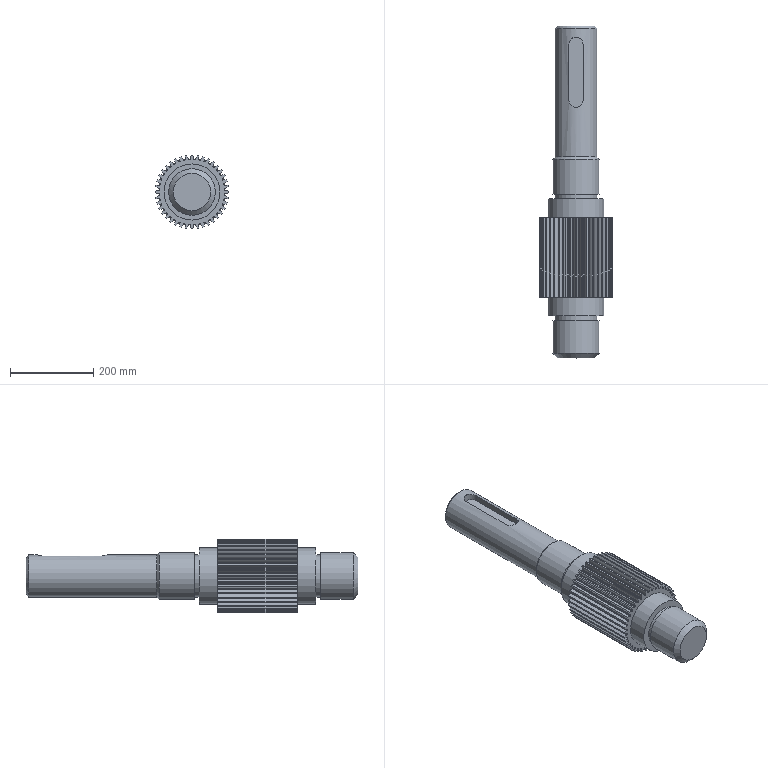Part | NX | features INSTANCE 15, BOSS 6, CHAMFER 6, Delete Body 3, SPLIT BODY 2, UNITE 2, BREP 1, CIRCULAR_ISET 1, CYLINDER 1, DATUM_CSYS 1, DATUM_PLANE 1, EXTRUDE 1, FSET 1, LINKED_BODY 1, MIRROR 1, MOVE_FACE 1, RECT_SLOT 1, SCALE 1, SKETCH 1, SYMBOLIC_THREAD 1, TRANSFORM_ISET 1 | 1 solid | 263 faces | volume 9920254 mm3 | spline 200 | cylinder 49 | plane 11 | cone 3 | commonest cylinder face diameters 158.203 x40 101.25 x3 33.75 x2 112.5 x2 135 x2